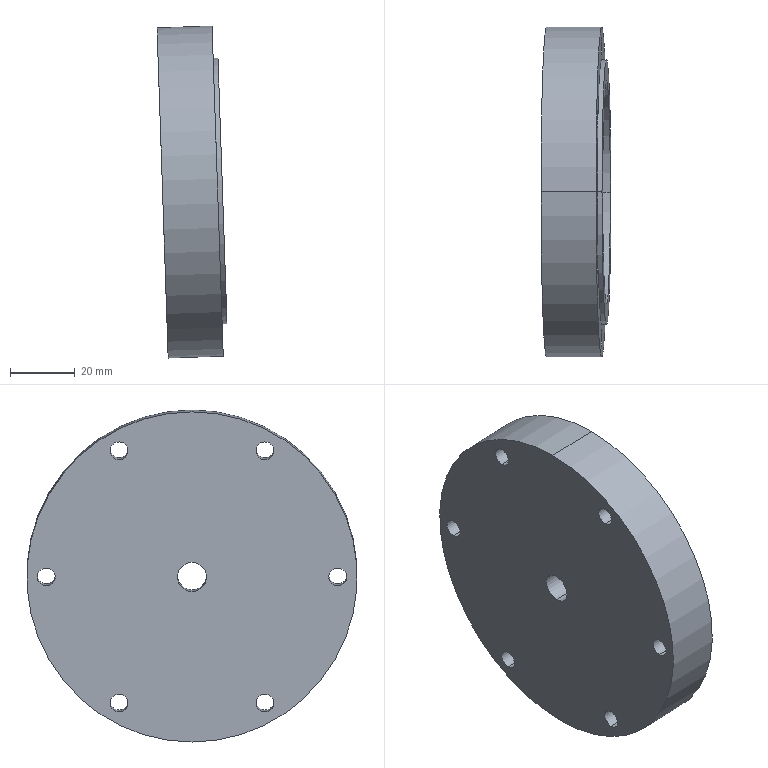Part | STEP file | 2026.6.15-Main Assembly图.sldasm-Part-132 | 1 solid | 24 faces | box 21.6 x 102 x 102.517 mm | volume 128530 mm3 | cylinder 20 | plane 4 | commonest cylinder face diameters 5.5 x12 9 x2 69 x2 82 x2 102 x2
STEP:
#1=CARTESIAN_POINT('',(-1475.055,735.086,4087.431));
#2=VERTEX_POINT('',#1);
#3=CARTESIAN_POINT('',(-1477.388,735.086,4156.392));
#4=VERTEX_POINT('',#3);
#5=CARTESIAN_POINT('',(-1476.221,735.086,4121.912));
#6=DIRECTION('',(-0.9994,0.,-0.03381));
#7=DIRECTION('',(-0.01691,0.866,0.4997));
#8=AXIS2_PLACEMENT_3D('',#5,#6,#7);
#9=CIRCLE('',#8,34.5);
#10=EDGE_CURVE('',#2,#4,#9,.T.);
#11=ORIENTED_EDGE('',*,*,#10,.F.);
#12=CARTESIAN_POINT('',(-1479.052,735.086,4087.296));
#13=VERTEX_POINT('',#12);
#14=CARTESIAN_POINT('',(-1475.055,735.086,4087.431));
#15=DIRECTION('',(-0.9994,0.,-0.03381));
#16=VECTOR('',#15,1000.);
#17=LINE('',#14,#16);
#18=EDGE_CURVE('',#2,#13,#17,.T.);
#19=ORIENTED_EDGE('',*,*,#18,.T.);
#20=CARTESIAN_POINT('',(-1481.386,735.086,4156.257));
#21=VERTEX_POINT('',#20);
#22=CARTESIAN_POINT('',(-1480.219,735.086,4121.776));
#23=DIRECTION('',(-0.9994,0.,-0.03381));
#24=DIRECTION('',(-0.01691,0.866,0.4997));
#25=AXIS2_PLACEMENT_3D('',#22,#23,#24);
#26=CIRCLE('',#25,34.5);
#27=EDGE_CURVE('',#13,#21,#26,.T.);
#28=ORIENTED_EDGE('',*,*,#27,.T.);
#29=CARTESIAN_POINT('',(-1477.388,735.086,4156.392));
#30=DIRECTION('',(-0.9994,0.,-0.03381));
#31=VECTOR('',#30,1000.);
#32=LINE('',#29,#31);
#33=EDGE_CURVE('',#4,#21,#32,.T.);
#34=ORIENTED_EDGE('',*,*,#33,.F.);
#35=EDGE_LOOP('',(#11,#19,#28,#34));
#36=FACE_OUTER_BOUND('',#35,.T.);
#37=CARTESIAN_POINT('',(-1476.221,735.086,4121.912));
#38=DIRECTION('',(-0.9994,0.,-0.03381));
#39=DIRECTION('',(-0.03381,0.,0.9994));
#40=AXIS2_PLACEMENT_3D('',#37,#38,#39);
#41=CYLINDRICAL_SURFACE('',#40,34.5);
#42=ADVANCED_FACE('',(#36),#41,.F.);
#43=CARTESIAN_POINT('',(-1477.608,735.086,4162.888));
#44=VERTEX_POINT('',#43);
#45=CARTESIAN_POINT('',(-1474.835,735.086,4080.935));
#46=VERTEX_POINT('',#45);
#47=CARTESIAN_POINT('',(-1476.221,735.086,4121.912));
#48=DIRECTION('',(-0.9994,0.,-0.03381));
#49=DIRECTION('',(-0.01691,0.866,0.4997));
#50=AXIS2_PLACEMENT_3D('',#47,#48,#49);
#51=CIRCLE('',#50,41.);
#52=EDGE_CURVE('',#44,#46,#51,.T.);
#53=ORIENTED_EDGE('',*,*,#52,.T.);
#54=CARTESIAN_POINT('',(-1476.334,735.086,4080.884));
#55=VERTEX_POINT('',#54);
#56=CARTESIAN_POINT('',(-1474.835,735.086,4080.935));
#57=DIRECTION('',(-0.9994,0.,-0.03381));
#58=VECTOR('',#57,1000.);
#59=LINE('',#56,#58);
#60=EDGE_CURVE('',#46,#55,#59,.T.);
#61=ORIENTED_EDGE('',*,*,#60,.T.);
#62=CARTESIAN_POINT('',(-1479.107,735.086,4162.837));
#63=VERTEX_POINT('',#62);
#64=CARTESIAN_POINT('',(-1477.72,735.086,4121.861));
#65=DIRECTION('',(-0.9994,0.,-0.03381));
#66=DIRECTION('',(-0.01691,0.866,0.4997));
#67=AXIS2_PLACEMENT_3D('',#64,#65,#66);
#68=CIRCLE('',#67,41.);
#69=EDGE_CURVE('',#63,#55,#68,.T.);
#70=ORIENTED_EDGE('',*,*,#69,.F.);
#71=CARTESIAN_POINT('',(-1477.608,735.086,4162.888));
#72=DIRECTION('',(-0.9994,0.,-0.03381));
#73=VECTOR('',#72,1000.);
#74=LINE('',#71,#73);
#75=EDGE_CURVE('',#44,#63,#74,.T.);
#76=ORIENTED_EDGE('',*,*,#75,.F.);
#77=EDGE_LOOP('',(#53,#61,#70,#76));
#78=FACE_OUTER_BOUND('',#77,.T.);
#79=CARTESIAN_POINT('',(-1476.221,735.086,4121.912));
#80=DIRECTION('',(-0.9994,0.,-0.03381));
#81=DIRECTION('',(-0.03381,0.,0.9994));
#82=AXIS2_PLACEMENT_3D('',#79,#80,#81);
#83=CYLINDRICAL_SURFACE('',#82,41.);
#84=ADVANCED_FACE('',(#78),#83,.T.);
#85=CARTESIAN_POINT('',(-1476.31,712.586,4080.164));
#86=VERTEX_POINT('',#85);
#87=CARTESIAN_POINT('',(-1476.496,712.586,4085.66));
#88=VERTEX_POINT('',#87);
#89=CARTESIAN_POINT('',(-1476.403,712.586,4082.912));
#90=DIRECTION('',(-0.9994,0.,-0.03381));
#91=DIRECTION('',(0.02928,0.5,-0.8655));
#92=AXIS2_PLACEMENT_3D('',#89,#90,#91);
#93=CIRCLE('',#92,2.75);
#94=EDGE_CURVE('',#86,#88,#93,.T.);
#95=ORIENTED_EDGE('',*,*,#94,.F.);
#96=CARTESIAN_POINT('',(-1493.3,712.586,4079.589));
#97=VERTEX_POINT('',#96);
#98=CARTESIAN_POINT('',(-1476.31,712.586,4080.164));
#99=DIRECTION('',(-0.9994,0.,-0.03381));
#100=VECTOR('',#99,1000.);
#101=LINE('',#98,#100);
#102=EDGE_CURVE('',#86,#97,#101,.T.);
#103=ORIENTED_EDGE('',*,*,#102,.T.);
#104=CARTESIAN_POINT('',(-1493.486,712.586,4085.086));
#105=VERTEX_POINT('',#104);
#106=CARTESIAN_POINT('',(-1493.393,712.586,4082.337));
#107=DIRECTION('',(-0.9994,0.,-0.03381));
#108=DIRECTION('',(0.02928,0.5,-0.8655));
#109=AXIS2_PLACEMENT_3D('',#106,#107,#108);
#110=CIRCLE('',#109,2.75);
#111=EDGE_CURVE('',#97,#105,#110,.T.);
#112=ORIENTED_EDGE('',*,*,#111,.T.);
#113=CARTESIAN_POINT('',(-1476.496,712.586,4085.66));
#114=DIRECTION('',(-0.9994,0.,-0.03381));
#115=VECTOR('',#114,1000.);
#116=LINE('',#113,#115);
#117=EDGE_CURVE('',#88,#105,#116,.T.);
#118=ORIENTED_EDGE('',*,*,#117,.F.);
#119=EDGE_LOOP('',(#95,#103,#112,#118));
#120=FACE_OUTER_BOUND('',#119,.T.);
#121=CARTESIAN_POINT('',(-1476.403,712.586,4082.912));
#122=DIRECTION('',(-0.9994,0.,-0.03381));
#123=DIRECTION('',(-0.03381,0.,0.9994));
#124=AXIS2_PLACEMENT_3D('',#121,#122,#123);
#125=CYLINDRICAL_SURFACE('',#124,2.75);
#126=ADVANCED_FACE('',(#120),#125,.F.);
#127=CARTESIAN_POINT('',(-1479.445,735.086,4172.832));
#128=VERTEX_POINT('',#127);
#129=CARTESIAN_POINT('',(-1475.996,735.086,4070.89));
#130=VERTEX_POINT('',#129);
#131=CARTESIAN_POINT('',(-1477.72,735.086,4121.861));
#132=DIRECTION('',(-0.9994,0.,-0.03381));
#133=DIRECTION('',(0.02928,0.5,-0.8655));
#134=AXIS2_PLACEMENT_3D('',#131,#132,#133);
#135=CIRCLE('',#134,51.);
#136=EDGE_CURVE('',#128,#130,#135,.T.);
#137=ORIENTED_EDGE('',*,*,#136,.T.);
#138=CARTESIAN_POINT('',(-1492.986,735.086,4070.315));
#139=VERTEX_POINT('',#138);
#140=CARTESIAN_POINT('',(-1475.996,735.086,4070.89));
#141=DIRECTION('',(-0.9994,0.,-0.03381));
#142=VECTOR('',#141,1000.);
#143=LINE('',#140,#142);
#144=EDGE_CURVE('',#130,#139,#143,.T.);
#145=ORIENTED_EDGE('',*,*,#144,.T.);
#146=CARTESIAN_POINT('',(-1496.435,735.086,4172.257));
#147=VERTEX_POINT('',#146);
#148=CARTESIAN_POINT('',(-1494.711,735.086,4121.286));
#149=DIRECTION('',(-0.9994,0.,-0.03381));
#150=DIRECTION('',(0.02928,0.5,-0.8655));
#151=AXIS2_PLACEMENT_3D('',#148,#149,#150);
#152=CIRCLE('',#151,51.);
#153=EDGE_CURVE('',#147,#139,#152,.T.);
#154=ORIENTED_EDGE('',*,*,#153,.F.);
#155=CARTESIAN_POINT('',(-1479.445,735.086,4172.832));
#156=DIRECTION('',(-0.9994,0.,-0.03381));
#157=VECTOR('',#156,1000.);
#158=LINE('',#155,#157);
#159=EDGE_CURVE('',#128,#147,#158,.T.);
#160=ORIENTED_EDGE('',*,*,#159,.F.);
#161=EDGE_LOOP('',(#137,#145,#154,#160));
#162=FACE_OUTER_BOUND('',#161,.T.);
#163=CARTESIAN_POINT('',(-1477.72,735.086,4121.861));
#164=DIRECTION('',(-0.9994,0.,-0.03381));
#165=DIRECTION('',(-0.03381,0.,0.9994));
#166=AXIS2_PLACEMENT_3D('',#163,#164,#165);
#167=CYLINDRICAL_SURFACE('',#166,51.);
#168=ADVANCED_FACE('',(#162),#167,.T.);
#169=CARTESIAN_POINT('',(-1478.945,757.586,4158.061));
#170=VERTEX_POINT('',#169);
#171=CARTESIAN_POINT('',(-1479.131,757.586,4163.558));
#172=VERTEX_POINT('',#171);
#173=CARTESIAN_POINT('',(-1479.038,757.586,4160.81));
#174=DIRECTION('',(-0.9994,0.,-0.03381));
#175=DIRECTION('',(0.02928,0.5,-0.8655));
#176=AXIS2_PLACEMENT_3D('',#173,#174,#175);
#177=CIRCLE('',#176,2.75);
#178=EDGE_CURVE('',#170,#172,#177,.T.);
#179=ORIENTED_EDGE('',*,*,#178,.F.);
#180=CARTESIAN_POINT('',(-1495.935,757.586,4157.486));
#181=VERTEX_POINT('',#180);
#182=CARTESIAN_POINT('',(-1478.945,757.586,4158.061));
#183=DIRECTION('',(-0.9994,0.,-0.03381));
#184=VECTOR('',#183,1000.);
#185=LINE('',#182,#184);
#186=EDGE_CURVE('',#170,#181,#185,.T.);
#187=ORIENTED_EDGE('',*,*,#186,.T.);
#188=CARTESIAN_POINT('',(-1496.121,757.586,4162.983));
#189=VERTEX_POINT('',#188);
#190=CARTESIAN_POINT('',(-1496.028,757.586,4160.235));
#191=DIRECTION('',(-0.9994,0.,-0.03381));
#192=DIRECTION('',(0.02928,0.5,-0.8655));
#193=AXIS2_PLACEMENT_3D('',#190,#191,#192);
#194=CIRCLE('',#193,2.75);
#195=EDGE_CURVE('',#181,#189,#194,.T.);
#196=ORIENTED_EDGE('',*,*,#195,.T.);
#197=CARTESIAN_POINT('',(-1479.131,757.586,4163.558));
#198=DIRECTION('',(-0.9994,0.,-0.03381));
#199=VECTOR('',#198,1000.);
#200=LINE('',#197,#199);
#201=EDGE_CURVE('',#172,#189,#200,.T.);
#202=ORIENTED_EDGE('',*,*,#201,.F.);
#203=EDGE_LOOP('',(#179,#187,#196,#202));
#204=FACE_OUTER_BOUND('',#203,.T.);
#205=CARTESIAN_POINT('',(-1479.038,757.586,4160.81));
#206=DIRECTION('',(-0.9994,0.,-0.03381));
#207=DIRECTION('',(-0.03381,0.,0.9994));
#208=AXIS2_PLACEMENT_3D('',#205,#206,#207);
#209=CYLINDRICAL_SURFACE('',#208,2.75);
#210=ADVANCED_FACE('',(#204),#209,.F.);
#211=CARTESIAN_POINT('',(-1478.945,712.586,4158.061));
#212=VERTEX_POINT('',#211);
#213=CARTESIAN_POINT('',(-1479.131,712.586,4163.558));
#214=VERTEX_POINT('',#213);
#215=CARTESIAN_POINT('',(-1479.038,712.586,4160.81));
#216=DIRECTION('',(-0.9994,0.,-0.03381));
#217=DIRECTION('',(0.02928,0.5,-0.8655));
#218=AXIS2_PLACEMENT_3D('',#215,#216,#217);
#219=CIRCLE('',#218,2.75);
#220=EDGE_CURVE('',#212,#214,#219,.T.);
#221=ORIENTED_EDGE('',*,*,#220,.F.);
#222=CARTESIAN_POINT('',(-1495.935,712.586,4157.486));
#223=VERTEX_POINT('',#222);
#224=CARTESIAN_POINT('',(-1478.945,712.586,4158.061));
#225=DIRECTION('',(-0.9994,0.,-0.03381));
#226=VECTOR('',#225,1000.);
#227=LINE('',#224,#226);
#228=EDGE_CURVE('',#212,#223,#227,.T.);
#229=ORIENTED_EDGE('',*,*,#228,.T.);
#230=CARTESIAN_POINT('',(-1496.121,712.586,4162.983));
#231=VERTEX_POINT('',#230);
#232=CARTESIAN_POINT('',(-1496.028,712.586,4160.235));
#233=DIRECTION('',(-0.9994,0.,-0.03381));
#234=DIRECTION('',(0.02928,0.5,-0.8655));
#235=AXIS2_PLACEMENT_3D('',#232,#233,#234);
#236=CIRCLE('',#235,2.75);
#237=EDGE_CURVE('',#223,#231,#236,.T.);
#238=ORIENTED_EDGE('',*,*,#237,.T.);
#239=CARTESIAN_POINT('',(-1479.131,712.586,4163.558));
#240=DIRECTION('',(-0.9994,0.,-0.03381));
#241=VECTOR('',#240,1000.);
#242=LINE('',#239,#241);
#243=EDGE_CURVE('',#214,#231,#242,.T.);
#244=ORIENTED_EDGE('',*,*,#243,.F.);
#245=EDGE_LOOP('',(#221,#229,#238,#244));
#246=FACE_OUTER_BOUND('',#245,.T.);
#247=CARTESIAN_POINT('',(-1479.038,712.586,4160.81));
#248=DIRECTION('',(-0.9994,0.,-0.03381));
#249=DIRECTION('',(-0.03381,0.,0.9994));
#250=AXIS2_PLACEMENT_3D('',#247,#248,#249);
#251=CYLINDRICAL_SURFACE('',#250,2.75);
#252=ADVANCED_FACE('',(#246),#251,.F.);
#253=CARTESIAN_POINT('',(-1477.627,780.086,4119.112));
#254=VERTEX_POINT('',#253);
#255=CARTESIAN_POINT('',(-1477.813,780.086,4124.609));
#256=VERTEX_POINT('',#255);
#257=CARTESIAN_POINT('',(-1477.72,780.086,4121.861));
#258=DIRECTION('',(-0.9994,0.,-0.03381));
#259=DIRECTION('',(0.02928,0.5,-0.8655));
#260=AXIS2_PLACEMENT_3D('',#257,#258,#259);
#261=CIRCLE('',#260,2.75);
#262=EDGE_CURVE('',#254,#256,#261,.T.);
#263=ORIENTED_EDGE('',*,*,#262,.F.);
#264=CARTESIAN_POINT('',(-1494.618,780.086,4118.538));
#265=VERTEX_POINT('',#264);
#266=CARTESIAN_POINT('',(-1477.627,780.086,4119.112));
#267=DIRECTION('',(-0.9994,0.,-0.03381));
#268=VECTOR('',#267,1000.);
#269=LINE('',#266,#268);
#270=EDGE_CURVE('',#254,#265,#269,.T.);
#271=ORIENTED_EDGE('',*,*,#270,.T.);
#272=CARTESIAN_POINT('',(-1494.804,780.086,4124.034));
#273=VERTEX_POINT('',#272);
#274=CARTESIAN_POINT('',(-1494.711,780.086,4121.286));
#275=DIRECTION('',(-0.9994,0.,-0.03381));
#276=DIRECTION('',(0.02928,0.5,-0.8655));
#277=AXIS2_PLACEMENT_3D('',#274,#275,#276);
#278=CIRCLE('',#277,2.75);
#279=EDGE_CURVE('',#265,#273,#278,.T.);
#280=ORIENTED_EDGE('',*,*,#279,.T.);
#281=CARTESIAN_POINT('',(-1477.813,780.086,4124.609));
#282=DIRECTION('',(-0.9994,0.,-0.03381));
#283=VECTOR('',#282,1000.);
#284=LINE('',#281,#283);
#285=EDGE_CURVE('',#256,#273,#284,.T.);
#286=ORIENTED_EDGE('',*,*,#285,.F.);
#287=EDGE_LOOP('',(#263,#271,#280,#286));
#288=FACE_OUTER_BOUND('',#287,.T.);
#289=CARTESIAN_POINT('',(-1477.72,780.086,4121.861));
#290=DIRECTION('',(-0.9994,0.,-0.03381));
#291=DIRECTION('',(-0.03381,0.,0.9994));
#292=AXIS2_PLACEMENT_3D('',#289,#290,#291);
#293=CYLINDRICAL_SURFACE('',#292,2.75);
#294=ADVANCED_FACE('',(#288),#293,.F.);
#295=CARTESIAN_POINT('',(-1477.627,690.086,4119.112));
#296=VERTEX_POINT('',#295);
#297=CARTESIAN_POINT('',(-1477.813,690.086,4124.609));
#298=VERTEX_POINT('',#297);
#299=CARTESIAN_POINT('',(-1477.72,690.086,4121.861));
#300=DIRECTION('',(-0.9994,0.,-0.03381));
#301=DIRECTION('',(0.02928,0.5,-0.8655));
#302=AXIS2_PLACEMENT_3D('',#299,#300,#301);
#303=CIRCLE('',#302,2.75);
#304=EDGE_CURVE('',#296,#298,#303,.T.);
#305=ORIENTED_EDGE('',*,*,#304,.F.);
#306=CARTESIAN_POINT('',(-1494.618,690.086,4118.538));
#307=VERTEX_POINT('',#306);
#308=CARTESIAN_POINT('',(-1477.627,690.086,4119.112));
#309=DIRECTION('',(-0.9994,0.,-0.03381));
#310=VECTOR('',#309,1000.);
#311=LINE('',#308,#310);
#312=EDGE_CURVE('',#296,#307,#311,.T.);
#313=ORIENTED_EDGE('',*,*,#312,.T.);
#314=CARTESIAN_POINT('',(-1494.804,690.086,4124.034));
#315=VERTEX_POINT('',#314);
#316=CARTESIAN_POINT('',(-1494.711,690.086,4121.286));
#317=DIRECTION('',(-0.9994,0.,-0.03381));
#318=DIRECTION('',(0.02928,0.5,-0.8655));
#319=AXIS2_PLACEMENT_3D('',#316,#317,#318);
#320=CIRCLE('',#319,2.75);
#321=EDGE_CURVE('',#307,#315,#320,.T.);
#322=ORIENTED_EDGE('',*,*,#321,.T.);
#323=CARTESIAN_POINT('',(-1477.813,690.086,4124.609));
#324=DIRECTION('',(-0.9994,0.,-0.03381));
#325=VECTOR('',#324,1000.);
#326=LINE('',#323,#325);
#327=EDGE_CURVE('',#298,#315,#326,.T.);
#328=ORIENTED_EDGE('',*,*,#327,.F.);
#329=EDGE_LOOP('',(#305,#313,#322,#328));
#330=FACE_OUTER_BOUND('',#329,.T.);
#331=CARTESIAN_POINT('',(-1477.72,690.086,4121.861));
#332=DIRECTION('',(-0.9994,0.,-0.03381));
#333=DIRECTION('',(-0.03381,0.,0.9994));
#334=AXIS2_PLACEMENT_3D('',#331,#332,#333);
#335=CYLINDRICAL_SURFACE('',#334,2.75);
#336=ADVANCED_FACE('',(#330),#335,.F.);
#337=CARTESIAN_POINT('',(-1480.067,735.086,4117.279));
#338=VERTEX_POINT('',#337);
#339=CARTESIAN_POINT('',(-1480.371,735.086,4126.274));
#340=VERTEX_POINT('',#339);
#341=CARTESIAN_POINT('',(-1480.219,735.086,4121.776));
#342=DIRECTION('',(-0.9994,0.,-0.03381));
#343=DIRECTION('',(0.02928,0.5,-0.8655));
#344=AXIS2_PLACEMENT_3D('',#341,#342,#343);
#345=CIRCLE('',#344,4.5);
#346=EDGE_CURVE('',#338,#340,#345,.T.);
#347=ORIENTED_EDGE('',*,*,#346,.F.);
#348=CARTESIAN_POINT('',(-1494.558,735.086,4116.789));
#349=VERTEX_POINT('',#348);
#350=CARTESIAN_POINT('',(-1477.568,735.086,4117.363));
#351=DIRECTION('',(-0.9994,0.,-0.03381));
#352=VECTOR('',#351,1000.);
#353=LINE('',#350,#352);
#354=EDGE_CURVE('',#338,#349,#353,.T.);
#355=ORIENTED_EDGE('',*,*,#354,.T.);
#356=CARTESIAN_POINT('',(-1494.863,735.086,4125.783));
#357=VERTEX_POINT('',#356);
#358=CARTESIAN_POINT('',(-1494.711,735.086,4121.286));
#359=DIRECTION('',(-0.9994,0.,-0.03381));
#360=DIRECTION('',(0.02928,0.5,-0.8655));
#361=AXIS2_PLACEMENT_3D('',#358,#359,#360);
#362=CIRCLE('',#361,4.5);
#363=EDGE_CURVE('',#349,#357,#362,.T.);
#364=ORIENTED_EDGE('',*,*,#363,.T.);
#365=CARTESIAN_POINT('',(-1477.873,735.086,4126.358));
#366=DIRECTION('',(-0.9994,0.,-0.03381));
#367=VECTOR('',#366,1000.);
#368=LINE('',#365,#367);
#369=EDGE_CURVE('',#340,#357,#368,.T.);
#370=ORIENTED_EDGE('',*,*,#369,.F.);
#371=EDGE_LOOP('',(#347,#355,#364,#370));
#372=FACE_OUTER_BOUND('',#371,.T.);
#373=CARTESIAN_POINT('',(-1477.72,735.086,4121.861));
#374=DIRECTION('',(-0.9994,0.,-0.03381));
#375=DIRECTION('',(-0.03381,0.,0.9994));
#376=AXIS2_PLACEMENT_3D('',#373,#374,#375);
#377=CYLINDRICAL_SURFACE('',#376,4.5);
#378=ADVANCED_FACE('',(#372),#377,.F.);
#379=CARTESIAN_POINT('',(-1476.31,757.586,4080.164));
#380=VERTEX_POINT('',#379);
#381=CARTESIAN_POINT('',(-1476.496,757.586,4085.66));
#382=VERTEX_POINT('',#381);
#383=CARTESIAN_POINT('',(-1476.403,757.586,4082.912));
#384=DIRECTION('',(-0.9994,0.,-0.03381));
#385=DIRECTION('',(0.02928,0.5,-0.8655));
#386=AXIS2_PLACEMENT_3D('',#383,#384,#385);
#387=CIRCLE('',#386,2.75);
#388=EDGE_CURVE('',#380,#382,#387,.T.);
#389=ORIENTED_EDGE('',*,*,#388,.F.);
#390=CARTESIAN_POINT('',(-1493.3,757.586,4079.589));
#391=VERTEX_POINT('',#390);
#392=CARTESIAN_POINT('',(-1476.31,757.586,4080.164));
#393=DIRECTION('',(-0.9994,0.,-0.03381));
#394=VECTOR('',#393,1000.);
#395=LINE('',#392,#394);
#396=EDGE_CURVE('',#380,#391,#395,.T.);
#397=ORIENTED_EDGE('',*,*,#396,.T.);
#398=CARTESIAN_POINT('',(-1493.486,757.586,4085.086));
#399=VERTEX_POINT('',#398);
#400=CARTESIAN_POINT('',(-1493.393,757.586,4082.337));
#401=DIRECTION('',(-0.9994,0.,-0.03381));
#402=DIRECTION('',(0.02928,0.5,-0.8655));
#403=AXIS2_PLACEMENT_3D('',#400,#401,#402);
#404=CIRCLE('',#403,2.75);
#405=EDGE_CURVE('',#391,#399,#404,.T.);
#406=ORIENTED_EDGE('',*,*,#405,.T.);
#407=CARTESIAN_POINT('',(-1476.496,757.586,4085.66));
#408=DIRECTION('',(-0.9994,0.,-0.03381));
#409=VECTOR('',#408,1000.);
#410=LINE('',#407,#409);
#411=EDGE_CURVE('',#382,#399,#410,.T.);
#412=ORIENTED_EDGE('',*,*,#411,.F.);
#413=EDGE_LOOP('',(#389,#397,#406,#412));
#414=FACE_OUTER_BOUND('',#413,.T.);
#415=CARTESIAN_POINT('',(-1476.403,757.586,4082.912));
#416=DIRECTION('',(-0.9994,0.,-0.03381));
#417=DIRECTION('',(-0.03381,0.,0.9994));
#418=AXIS2_PLACEMENT_3D('',#415,#416,#417);
#419=CYLINDRICAL_SURFACE('',#418,2.75);
#420=ADVANCED_FACE('',(#414),#419,.F.);
#421=CARTESIAN_POINT('',(-1480.219,735.086,4121.776));
#422=DIRECTION('',(-0.9994,0.,-0.03381));
#423=DIRECTION('',(0.02928,0.5,-0.8655));
#424=AXIS2_PLACEMENT_3D('',#421,#422,#423);
#425=CIRCLE('',#424,4.5);
#426=EDGE_CURVE('',#340,#338,#425,.T.);
#427=ORIENTED_EDGE('',*,*,#426,.T.);
#428=ORIENTED_EDGE('',*,*,#346,.T.);
#429=EDGE_LOOP('',(#427,#428));
#430=FACE_BOUND('',#429,.T.);
#431=CARTESIAN_POINT('',(-1480.219,735.086,4121.776));
#432=DIRECTION('',(-0.9994,0.,-0.03381));
#433=DIRECTION('',(-0.01691,0.866,0.4997));
#434=AXIS2_PLACEMENT_3D('',#431,#432,#433);
#435=CIRCLE('',#434,34.5);
#436=EDGE_CURVE('',#21,#13,#435,.T.);
#437=ORIENTED_EDGE('',*,*,#436,.F.);
#438=ORIENTED_EDGE('',*,*,#27,.F.);
#439=EDGE_LOOP('',(#437,#438));
#440=FACE_OUTER_BOUND('',#439,.T.);
#441=CARTESIAN_POINT('',(-1480.878,746.336,4141.251));
#442=DIRECTION('',(0.9994,0.,0.03381));
#443=DIRECTION('',(0.03381,0.,-0.9994));
#444=AXIS2_PLACEMENT_3D('',#441,#442,#443);
#445=PLANE('',#444);
#446=ADVANCED_FACE('',(#430,#440),#445,.T.);
#447=ORIENTED_EDGE('',*,*,#396,.F.);
#448=CARTESIAN_POINT('',(-1476.403,757.586,4082.912));
#449=DIRECTION('',(-0.9994,0.,-0.03381));
#450=DIRECTION('',(0.02928,0.5,-0.8655));
#451=AXIS2_PLACEMENT_3D('',#448,#449,#450);
#452=CIRCLE('',#451,2.75);
#453=EDGE_CURVE('',#382,#380,#452,.T.);
#454=ORIENTED_EDGE('',*,*,#453,.F.);
#455=ORIENTED_EDGE('',*,*,#411,.T.);
#456=CARTESIAN_POINT('',(-1493.393,757.586,4082.337));
#457=DIRECTION('',(-0.9994,0.,-0.03381));
#458=DIRECTION('',(0.02928,0.5,-0.8655));
#459=AXIS2_PLACEMENT_3D('',#456,#457,#458);
#460=CIRCLE('',#459,2.75);
#461=EDGE_CURVE('',#399,#391,#460,.T.);
#462=ORIENTED_EDGE('',*,*,#461,.T.);
#463=EDGE_LOOP('',(#447,#454,#455,#462));
#464=FACE_OUTER_BOUND('',#463,.T.);
#465=CARTESIAN_POINT('',(-1476.403,757.586,4082.912));
#466=DIRECTION('',(-0.9994,0.,-0.03381));
#467=DIRECTION('',(-0.03381,0.,0.9994));
#468=AXIS2_PLACEMENT_3D('',#465,#466,#467);
#469=CYLINDRICAL_SURFACE('',#468,2.75);
#470=ADVANCED_FACE('',(#464),#469,.F.);
#471=ORIENTED_EDGE('',*,*,#354,.F.);
#472=ORIENTED_EDGE('',*,*,#426,.F.);
#473=ORIENTED_EDGE('',*,*,#369,.T.);
#474=CARTESIAN_POINT('',(-1494.711,735.086,4121.286));
#475=DIRECTION('',(-0.9994,0.,-0.03381));
#476=DIRECTION('',(0.02928,0.5,-0.8655));
#477=AXIS2_PLACEMENT_3D('',#474,#475,#476);
#478=CIRCLE('',#477,4.5);
#479=EDGE_CURVE('',#357,#349,#478,.T.);
#480=ORIENTED_EDGE('',*,*,#479,.T.);
#481=EDGE_LOOP('',(#471,#472,#473,#480));
#482=FACE_OUTER_BOUND('',#481,.T.);
#483=CARTESIAN_POINT('',(-1477.72,735.086,4121.861));
#484=DIRECTION('',(-0.9994,0.,-0.03381));
#485=DIRECTION('',(-0.03381,0.,0.9994));
#486=AXIS2_PLACEMENT_3D('',#483,#484,#485);
#487=CYLINDRICAL_SURFACE('',#486,4.5);
#488=ADVANCED_FACE('',(#482),#487,.F.);
#489=ORIENTED_EDGE('',*,*,#312,.F.);
#490=CARTESIAN_POINT('',(-1477.72,690.086,4121.861));
#491=DIRECTION('',(-0.9994,0.,-0.03381));
#492=DIRECTION('',(0.02928,0.5,-0.8655));
#493=AXIS2_PLACEMENT_3D('',#490,#491,#492);
#494=CIRCLE('',#493,2.75);
#495=EDGE_CURVE('',#298,#296,#494,.T.);
#496=ORIENTED_EDGE('',*,*,#495,.F.);
#497=ORIENTED_EDGE('',*,*,#327,.T.);
#498=CARTESIAN_POINT('',(-1494.711,690.086,4121.286));
#499=DIRECTION('',(-0.9994,0.,-0.03381));
#500=DIRECTION('',(0.02928,0.5,-0.8655));
#501=AXIS2_PLACEMENT_3D('',#498,#499,#500);
#502=CIRCLE('',#501,2.75);
#503=EDGE_CURVE('',#315,#307,#502,.T.);
#504=ORIENTED_EDGE('',*,*,#503,.T.);
#505=EDGE_LOOP('',(#489,#496,#497,#504));
#506=FACE_OUTER_BOUND('',#505,.T.);
#507=CARTESIAN_POINT('',(-1477.72,690.086,4121.861));
#508=DIRECTION('',(-0.9994,0.,-0.03381));
#509=DIRECTION('',(-0.03381,0.,0.9994));
#510=AXIS2_PLACEMENT_3D('',#507,#508,#509);
#511=CYLINDRICAL_SURFACE('',#510,2.75);
#512=ADVANCED_FACE('',(#506),#511,.F.);
#513=ORIENTED_EDGE('',*,*,#270,.F.);
#514=CARTESIAN_POINT('',(-1477.72,780.086,4121.861));
#515=DIRECTION('',(-0.9994,0.,-0.03381));
#516=DIRECTION('',(0.02928,0.5,-0.8655));
#517=AXIS2_PLACEMENT_3D('',#514,#515,#516);
#518=CIRCLE('',#517,2.75);
#519=EDGE_CURVE('',#256,#254,#518,.T.);
#520=ORIENTED_EDGE('',*,*,#519,.F.);
#521=ORIENTED_EDGE('',*,*,#285,.T.);
#522=CARTESIAN_POINT('',(-1494.711,780.086,4121.286));
#523=DIRECTION('',(-0.9994,0.,-0.03381));
#524=DIRECTION('',(0.02928,0.5,-0.8655));
#525=AXIS2_PLACEMENT_3D('',#522,#523,#524);
#526=CIRCLE('',#525,2.75);
#527=EDGE_CURVE('',#273,#265,#526,.T.);
#528=ORIENTED_EDGE('',*,*,#527,.T.);
#529=EDGE_LOOP('',(#513,#520,#521,#528));
#530=FACE_OUTER_BOUND('',#529,.T.);
#531=CARTESIAN_POINT('',(-1477.72,780.086,4121.861));
#532=DIRECTION('',(-0.9994,0.,-0.03381));
#533=DIRECTION('',(-0.03381,0.,0.9994));
#534=AXIS2_PLACEMENT_3D('',#531,#532,#533);
#535=CYLINDRICAL_SURFACE('',#534,2.75);
#536=ADVANCED_FACE('',(#530),#535,.F.);
#537=ORIENTED_EDGE('',*,*,#228,.F.);
#538=CARTESIAN_POINT('',(-1479.038,712.586,4160.81));
#539=DIRECTION('',(-0.9994,0.,-0.03381));
#540=DIRECTION('',(0.02928,0.5,-0.8655));
#541=AXIS2_PLACEMENT_3D('',#538,#539,#540);
#542=CIRCLE('',#541,2.75);
#543=EDGE_CURVE('',#214,#212,#542,.T.);
#544=ORIENTED_EDGE('',*,*,#543,.F.);
#545=ORIENTED_EDGE('',*,*,#243,.T.);
#546=CARTESIAN_POINT('',(-1496.028,712.586,4160.235));
#547=DIRECTION('',(-0.9994,0.,-0.03381));
#548=DIRECTION('',(0.02928,0.5,-0.8655));
#549=AXIS2_PLACEMENT_3D('',#546,#547,#548);
#550=CIRCLE('',#549,2.75);
#551=EDGE_CURVE('',#231,#223,#550,.T.);
#552=ORIENTED_EDGE('',*,*,#551,.T.);
#553=EDGE_LOOP('',(#537,#544,#545,#552));
#554=FACE_OUTER_BOUND('',#553,.T.);
#555=CARTESIAN_POINT('',(-1479.038,712.586,4160.81));
#556=DIRECTION('',(-0.9994,0.,-0.03381));
#557=DIRECTION('',(-0.03381,0.,0.9994));
#558=AXIS2_PLACEMENT_3D('',#555,#556,#557);
#559=CYLINDRICAL_SURFACE('',#558,2.75);
#560=ADVANCED_FACE('',(#554),#559,.F.);
#561=ORIENTED_EDGE('',*,*,#186,.F.);
#562=CARTESIAN_POINT('',(-1479.038,757.586,4160.81));
#563=DIRECTION('',(-0.9994,0.,-0.03381));
#564=DIRECTION('',(0.02928,0.5,-0.8655));
#565=AXIS2_PLACEMENT_3D('',#562,#563,#564);
#566=CIRCLE('',#565,2.75);
#567=EDGE_CURVE('',#172,#170,#566,.T.);
#568=ORIENTED_EDGE('',*,*,#567,.F.);
#569=ORIENTED_EDGE('',*,*,#201,.T.);
#570=CARTESIAN_POINT('',(-1496.028,757.586,4160.235));
#571=DIRECTION('',(-0.9994,0.,-0.03381));
#572=DIRECTION('',(0.02928,0.5,-0.8655));
#573=AXIS2_PLACEMENT_3D('',#570,#571,#572);
#574=CIRCLE('',#573,2.75);
#575=EDGE_CURVE('',#189,#181,#574,.T.);
#576=ORIENTED_EDGE('',*,*,#575,.T.);
#577=EDGE_LOOP('',(#561,#568,#569,#576));
#578=FACE_OUTER_BOUND('',#577,.T.);
#579=CARTESIAN_POINT('',(-1479.038,757.586,4160.81));
#580=DIRECTION('',(-0.9994,0.,-0.03381));
#581=DIRECTION('',(-0.03381,0.,0.9994));
#582=AXIS2_PLACEMENT_3D('',#579,#580,#581);
#583=CYLINDRICAL_SURFACE('',#582,2.75);
#584=ADVANCED_FACE('',(#578),#583,.F.);
#585=ORIENTED_EDGE('',*,*,#144,.F.);
#586=CARTESIAN_POINT('',(-1477.72,735.086,4121.861));
#587=DIRECTION('',(-0.9994,0.,-0.03381));
#588=DIRECTION('',(0.02928,0.5,-0.8655));
#589=AXIS2_PLACEMENT_3D('',#586,#587,#588);
#590=CIRCLE('',#589,51.);
#591=EDGE_CURVE('',#130,#128,#590,.T.);
#592=ORIENTED_EDGE('',*,*,#591,.T.);
#593=ORIENTED_EDGE('',*,*,#159,.T.);
#594=CARTESIAN_POINT('',(-1494.711,735.086,4121.286));
#595=DIRECTION('',(-0.9994,0.,-0.03381));
#596=DIRECTION('',(0.02928,0.5,-0.8655));
#597=AXIS2_PLACEMENT_3D('',#594,#595,#596);
#598=CIRCLE('',#597,51.);
#599=EDGE_CURVE('',#139,#147,#598,.T.);
#600=ORIENTED_EDGE('',*,*,#599,.F.);
#601=EDGE_LOOP('',(#585,#592,#593,#600));
#602=FACE_OUTER_BOUND('',#601,.T.);
#603=CARTESIAN_POINT('',(-1477.72,735.086,4121.861));
#604=DIRECTION('',(-0.9994,0.,-0.03381));
#605=DIRECTION('',(-0.03381,0.,0.9994));
#606=AXIS2_PLACEMENT_3D('',#603,#604,#605);
#607=CYLINDRICAL_SURFACE('',#606,51.);
#608=ADVANCED_FACE('',(#602),#607,.T.);
#609=ORIENTED_EDGE('',*,*,#102,.F.);
#610=CARTESIAN_POINT('',(-1476.403,712.586,4082.912));
#611=DIRECTION('',(-0.9994,0.,-0.03381));
#612=DIRECTION('',(0.02928,0.5,-0.8655));
#613=AXIS2_PLACEMENT_3D('',#610,#611,#612);
#614=CIRCLE('',#613,2.75);
#615=EDGE_CURVE('',#88,#86,#614,.T.);
#616=ORIENTED_EDGE('',*,*,#615,.F.);
#617=ORIENTED_EDGE('',*,*,#117,.T.);
#618=CARTESIAN_POINT('',(-1493.393,712.586,4082.337));
#619=DIRECTION('',(-0.9994,0.,-0.03381));
#620=DIRECTION('',(0.02928,0.5,-0.8655));
#621=AXIS2_PLACEMENT_3D('',#618,#619,#620);
#622=CIRCLE('',#621,2.75);
#623=EDGE_CURVE('',#105,#97,#622,.T.);
#624=ORIENTED_EDGE('',*,*,#623,.T.);
#625=EDGE_LOOP('',(#609,#616,#617,#624));
#626=FACE_OUTER_BOUND('',#625,.T.);
#627=CARTESIAN_POINT('',(-1476.403,712.586,4082.912));
#628=DIRECTION('',(-0.9994,0.,-0.03381));
#629=DIRECTION('',(-0.03381,0.,0.9994));
#630=AXIS2_PLACEMENT_3D('',#627,#628,#629);
#631=CYLINDRICAL_SURFACE('',#630,2.75);
#632=ADVANCED_FACE('',(#626),#631,.F.);
#633=ORIENTED_EDGE('',*,*,#69,.T.);
#634=CARTESIAN_POINT('',(-1477.72,735.086,4121.861));
#635=DIRECTION('',(-0.9994,0.,-0.03381));
#636=DIRECTION('',(-0.01691,0.866,0.4997));
#637=AXIS2_PLACEMENT_3D('',#634,#635,#636);
#638=CIRCLE('',#637,41.);
#639=EDGE_CURVE('',#55,#63,#638,.T.);
#640=ORIENTED_EDGE('',*,*,#639,.T.);
#641=EDGE_LOOP('',(#633,#640));
#642=FACE_BOUND('',#641,.T.);
#643=ORIENTED_EDGE('',*,*,#136,.F.);
#644=ORIENTED_EDGE('',*,*,#591,.F.);
#645=EDGE_LOOP('',(#643,#644));
#646=FACE_OUTER_BOUND('',#645,.T.);
#647=ORIENTED_EDGE('',*,*,#567,.T.);
#648=ORIENTED_EDGE('',*,*,#178,.T.);
#649=EDGE_LOOP('',(#647,#648));
#650=FACE_BOUND('',#649,.T.);
#651=ORIENTED_EDGE('',*,*,#543,.T.);
#652=ORIENTED_EDGE('',*,*,#220,.T.);
#653=EDGE_LOOP('',(#651,#652));
#654=FACE_BOUND('',#653,.T.);
#655=ORIENTED_EDGE('',*,*,#519,.T.);
#656=ORIENTED_EDGE('',*,*,#262,.T.);
#657=EDGE_LOOP('',(#655,#656));
#658=FACE_BOUND('',#657,.T.);
#659=ORIENTED_EDGE('',*,*,#495,.T.);
#660=ORIENTED_EDGE('',*,*,#304,.T.);
#661=EDGE_LOOP('',(#659,#660));
#662=FACE_BOUND('',#661,.T.);
#663=ORIENTED_EDGE('',*,*,#453,.T.);
#664=ORIENTED_EDGE('',*,*,#388,.T.);
#665=EDGE_LOOP('',(#663,#664));
#666=FACE_BOUND('',#665,.T.);
#667=ORIENTED_EDGE('',*,*,#615,.T.);
#668=ORIENTED_EDGE('',*,*,#94,.T.);
#669=EDGE_LOOP('',(#667,#668));
#670=FACE_BOUND('',#669,.T.);
#671=CARTESIAN_POINT('',(-1478.379,746.336,4141.335));
#672=DIRECTION('',(0.9994,0.,0.03381));
#673=DIRECTION('',(0.03381,0.,-0.9994));
#674=AXIS2_PLACEMENT_3D('',#671,#672,#673);
#675=PLANE('',#674);
#676=ADVANCED_FACE('',(#642,#646,#650,#654,#658,#662,#666,#670),#675,.T.);
#677=ORIENTED_EDGE('',*,*,#153,.T.);
#678=ORIENTED_EDGE('',*,*,#599,.T.);
#679=EDGE_LOOP('',(#677,#678));
#680=FACE_OUTER_BOUND('',#679,.T.);
#681=ORIENTED_EDGE('',*,*,#575,.F.);
#682=ORIENTED_EDGE('',*,*,#195,.F.);
#683=EDGE_LOOP('',(#681,#682));
#684=FACE_BOUND('',#683,.T.);
#685=ORIENTED_EDGE('',*,*,#551,.F.);
#686=ORIENTED_EDGE('',*,*,#237,.F.);
#687=EDGE_LOOP('',(#685,#686));
#688=FACE_BOUND('',#687,.T.);
#689=ORIENTED_EDGE('',*,*,#527,.F.);
#690=ORIENTED_EDGE('',*,*,#279,.F.);
#691=EDGE_LOOP('',(#689,#690));
#692=FACE_BOUND('',#691,.T.);
#693=ORIENTED_EDGE('',*,*,#503,.F.);
#694=ORIENTED_EDGE('',*,*,#321,.F.);
#695=EDGE_LOOP('',(#693,#694));
#696=FACE_BOUND('',#695,.T.);
#697=ORIENTED_EDGE('',*,*,#479,.F.);
#698=ORIENTED_EDGE('',*,*,#363,.F.);
#699=EDGE_LOOP('',(#697,#698));
#700=FACE_BOUND('',#699,.T.);
#701=ORIENTED_EDGE('',*,*,#461,.F.);
#702=ORIENTED_EDGE('',*,*,#405,.F.);
#703=EDGE_LOOP('',(#701,#702));
#704=FACE_BOUND('',#703,.T.);
#705=ORIENTED_EDGE('',*,*,#623,.F.);
#706=ORIENTED_EDGE('',*,*,#111,.F.);
#707=EDGE_LOOP('',(#705,#706));
#708=FACE_BOUND('',#707,.T.);
#709=CARTESIAN_POINT('',(-1495.37,746.336,4140.76));
#710=DIRECTION('',(0.9994,0.,0.03381));
#711=DIRECTION('',(0.03381,0.,-0.9994));
#712=AXIS2_PLACEMENT_3D('',#709,#710,#711);
#713=PLANE('',#712);
#714=ADVANCED_FACE('',(#680,#684,#688,#692,#696,#700,#704,#708),#713,.F.);
#715=ORIENTED_EDGE('',*,*,#60,.F.);
#716=CARTESIAN_POINT('',(-1476.221,735.086,4121.912));
#717=DIRECTION('',(-0.9994,0.,-0.03381));
#718=DIRECTION('',(-0.01691,0.866,0.4997));
#719=AXIS2_PLACEMENT_3D('',#716,#717,#718);
#720=CIRCLE('',#719,41.);
#721=EDGE_CURVE('',#46,#44,#720,.T.);
#722=ORIENTED_EDGE('',*,*,#721,.T.);
#723=ORIENTED_EDGE('',*,*,#75,.T.);
#724=ORIENTED_EDGE('',*,*,#639,.F.);
#725=EDGE_LOOP('',(#715,#722,#723,#724));
#726=FACE_OUTER_BOUND('',#725,.T.);
#727=CARTESIAN_POINT('',(-1476.221,735.086,4121.912));
#728=DIRECTION('',(-0.9994,0.,-0.03381));
#729=DIRECTION('',(-0.03381,0.,0.9994));
#730=AXIS2_PLACEMENT_3D('',#727,#728,#729);
#731=CYLINDRICAL_SURFACE('',#730,41.);
#732=ADVANCED_FACE('',(#726),#731,.T.);
#733=ORIENTED_EDGE('',*,*,#18,.F.);
#734=CARTESIAN_POINT('',(-1476.221,735.086,4121.912));
#735=DIRECTION('',(-0.9994,0.,-0.03381));
#736=DIRECTION('',(-0.01691,0.866,0.4997));
#737=AXIS2_PLACEMENT_3D('',#734,#735,#736);
#738=CIRCLE('',#737,34.5);
#739=EDGE_CURVE('',#4,#2,#738,.T.);
#740=ORIENTED_EDGE('',*,*,#739,.F.);
#741=ORIENTED_EDGE('',*,*,#33,.T.);
#742=ORIENTED_EDGE('',*,*,#436,.T.);
#743=EDGE_LOOP('',(#733,#740,#741,#742));
#744=FACE_OUTER_BOUND('',#743,.T.);
#745=CARTESIAN_POINT('',(-1476.221,735.086,4121.912));
#746=DIRECTION('',(-0.9994,0.,-0.03381));
#747=DIRECTION('',(-0.03381,0.,0.9994));
#748=AXIS2_PLACEMENT_3D('',#745,#746,#747);
#749=CYLINDRICAL_SURFACE('',#748,34.5);
#750=ADVANCED_FACE('',(#744),#749,.F.);
#751=ORIENTED_EDGE('',*,*,#52,.F.);
#752=ORIENTED_EDGE('',*,*,#721,.F.);
#753=EDGE_LOOP('',(#751,#752));
#754=FACE_OUTER_BOUND('',#753,.T.);
#755=ORIENTED_EDGE('',*,*,#739,.T.);
#756=ORIENTED_EDGE('',*,*,#10,.T.);
#757=EDGE_LOOP('',(#755,#756));
#758=FACE_BOUND('',#757,.T.);
#759=CARTESIAN_POINT('',(-1476.221,735.086,4121.912));
#760=DIRECTION('',(0.9994,0.,0.03381));
#761=DIRECTION('',(0.03381,0.,-0.9994));
#762=AXIS2_PLACEMENT_3D('',#759,#760,#761);
#763=PLANE('',#762);
#764=ADVANCED_FACE('',(#754,#758),#763,.T.);
#765=CLOSED_SHELL('',(#42,#84,#126,#168,#210,#252,#294,#336,#378,#420,#446,#470,#488,#512,#536,#560,#584,#608,#632,#676,#714,#732,#750,#764));
#766=MANIFOLD_SOLID_BREP('',#765);
#767=CARTESIAN_POINT('',(0.,0.,0.));
#768=DIRECTION('',(0.,0.,1.));
#769=DIRECTION('',(1.,0.,0.));
#770=AXIS2_PLACEMENT_3D('',#767,#768,#769);
#771=(LENGTH_UNIT()NAMED_UNIT(*)SI_UNIT(.MILLI.,.METRE.));
#772=UNCERTAINTY_MEASURE_WITH_UNIT(LENGTH_MEASURE(0.00001),#771,'','');
#773=(NAMED_UNIT(*)PLANE_ANGLE_UNIT()SI_UNIT($,.RADIAN.));
#774=(NAMED_UNIT(*)SI_UNIT($,.STERADIAN.)SOLID_ANGLE_UNIT());
#775=(GEOMETRIC_REPRESENTATION_CONTEXT(3)GLOBAL_UNCERTAINTY_ASSIGNED_CONTEXT((#772))GLOBAL_UNIT_ASSIGNED_CONTEXT((#771,#773,#774))REPRESENTATION_CONTEXT('',''));
#776=ADVANCED_BREP_SHAPE_REPRESENTATION('',(#766,#770),#775);